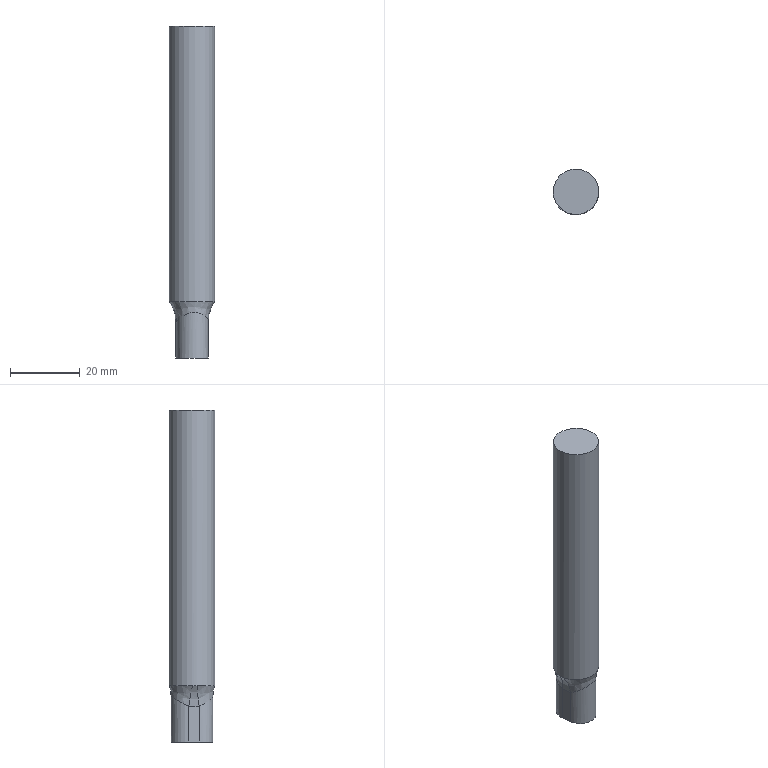Part | NX | features SPES-C 13-10-12.00-9.000 2 | 1 solid | 11 faces | box 13 x 13 x 95 mm | volume 11996 mm3 | plane 4 | spline 4 | cylinder 3 | commonest cylinder face diameters 9 x2 13 x1
STEP:
#1=CARTESIAN_POINT('',(601.161,-36.407,-10.773));
#2=VERTEX_POINT('',#1);
#3=CARTESIAN_POINT('',(601.161,-36.407,-21.));
#4=VERTEX_POINT('',#3);
#5=CARTESIAN_POINT('',(601.161,-36.407,-4.878));
#6=DIRECTION('',(0.,0.,-1.));
#7=VECTOR('',#6,1000.);
#8=LINE('',#5,#7);
#9=EDGE_CURVE('',#2,#4,#8,.T.);
#10=ORIENTED_EDGE('',*,*,#9,.F.);
#11=CARTESIAN_POINT('',(610.092,-35.294,-10.773));
#12=VERTEX_POINT('',#11);
#13=CARTESIAN_POINT('',(601.161,-36.407,-10.773));
#14=CARTESIAN_POINT('',(601.016,-35.246,-10.241));
#15=CARTESIAN_POINT('',(601.492,-33.509,-9.332));
#16=CARTESIAN_POINT('',(603.219,-31.901,-8.27));
#17=CARTESIAN_POINT('',(605.065,-31.242,-7.864));
#18=CARTESIAN_POINT('',(606.998,-31.435,-8.274));
#19=CARTESIAN_POINT('',(609.066,-32.573,-9.336));
#20=CARTESIAN_POINT('',(609.947,-34.134,-10.242));
#21=CARTESIAN_POINT('',(610.092,-35.294,-10.773));
#22=B_SPLINE_CURVE_WITH_KNOTS('',3,(#13,#14,#15,#16,#17,#18,#19,#20,#21),.UNSPECIFIED.,.F.,.F.,(4,1,1,1,1,1,4),(0.,0.003836,0.005754,0.007673,0.009591,0.01151,0.01535),.UNSPECIFIED.);
#23=EDGE_CURVE('',#2,#12,#22,.T.);
#24=ORIENTED_EDGE('',*,*,#23,.T.);
#25=CARTESIAN_POINT('',(610.092,-35.294,-21.));
#26=VERTEX_POINT('',#25);
#27=CARTESIAN_POINT('',(610.092,-35.294,-4.878));
#28=DIRECTION('',(0.,0.,-1.));
#29=VECTOR('',#28,1000.);
#30=LINE('',#27,#29);
#31=EDGE_CURVE('',#12,#26,#30,.T.);
#32=ORIENTED_EDGE('',*,*,#31,.T.);
#33=CARTESIAN_POINT('',(605.626,-35.851,-21.));
#34=DIRECTION('',(0.,0.,1.));
#35=DIRECTION('',(1.,0.,0.));
#36=AXIS2_PLACEMENT_3D('',#33,#34,#35);
#37=CIRCLE('',#36,4.5);
#38=EDGE_CURVE('',#26,#4,#37,.T.);
#39=ORIENTED_EDGE('',*,*,#38,.T.);
#40=EDGE_LOOP('',(#10,#24,#32,#39));
#41=FACE_BOUND('',#40,.T.);
#42=CARTESIAN_POINT('',(605.626,-35.851,-4.878));
#43=DIRECTION('',(0.,0.,-1.));
#44=DIRECTION('',(-1.,0.,0.));
#45=AXIS2_PLACEMENT_3D('',#42,#43,#44);
#46=CYLINDRICAL_SURFACE('',#45,4.5);
#47=ADVANCED_FACE('',(#41),#46,.T.);
#48=CARTESIAN_POINT('',(601.531,-39.384,-10.773));
#49=VERTEX_POINT('',#48);
#50=CARTESIAN_POINT('',(601.531,-39.384,-21.));
#51=VERTEX_POINT('',#50);
#52=CARTESIAN_POINT('',(601.531,-39.384,-4.878));
#53=DIRECTION('',(0.,0.,-1.));
#54=VECTOR('',#53,1000.);
#55=LINE('',#52,#54);
#56=EDGE_CURVE('',#49,#51,#55,.T.);
#57=ORIENTED_EDGE('',*,*,#56,.F.);
#58=CARTESIAN_POINT('',(601.531,-39.384,-10.773));
#59=CARTESIAN_POINT('',(601.408,-38.394,-10.914));
#60=CARTESIAN_POINT('',(601.284,-37.397,-10.914));
#61=CARTESIAN_POINT('',(601.161,-36.407,-10.773));
#62=B_SPLINE_CURVE_WITH_KNOTS('',3,(#58,#59,#60,#61),.UNSPECIFIED.,.F.,.F.,(4,4),(0.,0.003022),.UNSPECIFIED.);
#63=EDGE_CURVE('',#49,#2,#62,.T.);
#64=ORIENTED_EDGE('',*,*,#63,.T.);
#65=ORIENTED_EDGE('',*,*,#9,.T.);
#66=CARTESIAN_POINT('',(601.531,-39.384,-21.));
#67=DIRECTION('',(-0.1236,0.9923,0.));
#68=VECTOR('',#67,1000.);
#69=LINE('',#66,#68);
#70=EDGE_CURVE('',#51,#4,#69,.T.);
#71=ORIENTED_EDGE('',*,*,#70,.F.);
#72=EDGE_LOOP('',(#57,#64,#65,#71));
#73=FACE_BOUND('',#72,.T.);
#74=CARTESIAN_POINT('',(601.531,-39.384,-4.878));
#75=DIRECTION('',(-0.9923,-0.1236,0.));
#76=DIRECTION('',(0.1236,-0.9923,0.));
#77=AXIS2_PLACEMENT_3D('',#74,#75,#76);
#78=PLANE('',#77);
#79=ADVANCED_FACE('',(#73),#78,.T.);
#80=CARTESIAN_POINT('',(610.462,-38.271,-10.773));
#81=VERTEX_POINT('',#80);
#82=CARTESIAN_POINT('',(610.462,-38.271,-21.));
#83=VERTEX_POINT('',#82);
#84=CARTESIAN_POINT('',(610.462,-38.271,-4.878));
#85=DIRECTION('',(0.,0.,-1.));
#86=VECTOR('',#85,1000.);
#87=LINE('',#84,#86);
#88=EDGE_CURVE('',#81,#83,#87,.T.);
#89=ORIENTED_EDGE('',*,*,#88,.F.);
#90=CARTESIAN_POINT('',(610.462,-38.271,-10.773));
#91=CARTESIAN_POINT('',(610.607,-39.433,-10.241));
#92=CARTESIAN_POINT('',(610.131,-41.169,-9.332));
#93=CARTESIAN_POINT('',(608.404,-42.778,-8.27));
#94=CARTESIAN_POINT('',(606.559,-43.436,-7.864));
#95=CARTESIAN_POINT('',(604.625,-43.244,-8.274));
#96=CARTESIAN_POINT('',(602.557,-42.106,-9.336));
#97=CARTESIAN_POINT('',(601.676,-40.544,-10.242));
#98=CARTESIAN_POINT('',(601.531,-39.384,-10.773));
#99=B_SPLINE_CURVE_WITH_KNOTS('',3,(#90,#91,#92,#93,#94,#95,#96,#97,#98),.UNSPECIFIED.,.F.,.F.,(4,1,1,1,1,1,4),(0.,0.003836,0.005754,0.007673,0.009591,0.01151,0.01535),.UNSPECIFIED.);
#100=EDGE_CURVE('',#81,#49,#99,.T.);
#101=ORIENTED_EDGE('',*,*,#100,.T.);
#102=ORIENTED_EDGE('',*,*,#56,.T.);
#103=CARTESIAN_POINT('',(605.997,-38.828,-21.));
#104=DIRECTION('',(0.,0.,1.));
#105=DIRECTION('',(1.,0.,0.));
#106=AXIS2_PLACEMENT_3D('',#103,#104,#105);
#107=CIRCLE('',#106,4.5);
#108=EDGE_CURVE('',#51,#83,#107,.T.);
#109=ORIENTED_EDGE('',*,*,#108,.T.);
#110=EDGE_LOOP('',(#89,#101,#102,#109));
#111=FACE_BOUND('',#110,.T.);
#112=CARTESIAN_POINT('',(605.997,-38.828,-4.878));
#113=DIRECTION('',(0.,0.,-1.));
#114=DIRECTION('',(-1.,0.,0.));
#115=AXIS2_PLACEMENT_3D('',#112,#113,#114);
#116=CYLINDRICAL_SURFACE('',#115,4.5);
#117=ADVANCED_FACE('',(#111),#116,.T.);
#118=ORIENTED_EDGE('',*,*,#31,.F.);
#119=CARTESIAN_POINT('',(610.092,-35.294,-10.773));
#120=CARTESIAN_POINT('',(610.215,-36.284,-10.914));
#121=CARTESIAN_POINT('',(610.339,-37.281,-10.914));
#122=CARTESIAN_POINT('',(610.462,-38.271,-10.773));
#123=B_SPLINE_CURVE_WITH_KNOTS('',3,(#119,#120,#121,#122),.UNSPECIFIED.,.F.,.F.,(4,4),(0.,0.003022),.UNSPECIFIED.);
#124=EDGE_CURVE('',#12,#81,#123,.T.);
#125=ORIENTED_EDGE('',*,*,#124,.T.);
#126=ORIENTED_EDGE('',*,*,#88,.T.);
#127=CARTESIAN_POINT('',(610.462,-38.271,-21.));
#128=DIRECTION('',(-0.1236,0.9923,0.));
#129=VECTOR('',#128,1000.);
#130=LINE('',#127,#129);
#131=EDGE_CURVE('',#83,#26,#130,.T.);
#132=ORIENTED_EDGE('',*,*,#131,.T.);
#133=EDGE_LOOP('',(#118,#125,#126,#132));
#134=FACE_BOUND('',#133,.T.);
#135=CARTESIAN_POINT('',(610.462,-38.271,-4.878));
#136=DIRECTION('',(-0.9923,-0.1236,0.));
#137=DIRECTION('',(0.1236,-0.9923,0.));
#138=AXIS2_PLACEMENT_3D('',#135,#136,#137);
#139=PLANE('',#138);
#140=ADVANCED_FACE('',(#134),#139,.F.);
#141=ORIENTED_EDGE('',*,*,#38,.F.);
#142=ORIENTED_EDGE('',*,*,#131,.F.);
#143=ORIENTED_EDGE('',*,*,#108,.F.);
#144=ORIENTED_EDGE('',*,*,#70,.T.);
#145=EDGE_LOOP('',(#141,#142,#143,#144));
#146=FACE_BOUND('',#145,.T.);
#147=CARTESIAN_POINT('',(605.626,-35.851,-21.));
#148=DIRECTION('',(0.,0.,1.));
#149=DIRECTION('',(1.,0.,0.));
#150=AXIS2_PLACEMENT_3D('',#147,#148,#149);
#151=PLANE('',#150);
#152=ADVANCED_FACE('',(#146),#151,.F.);
#153=CARTESIAN_POINT('',(599.312,-37.339,74.));
#154=VERTEX_POINT('',#153);
#155=CARTESIAN_POINT('',(605.812,-37.339,74.));
#156=DIRECTION('',(0.,0.,-1.));
#157=DIRECTION('',(-1.,0.,0.));
#158=AXIS2_PLACEMENT_3D('',#155,#156,#157);
#159=CIRCLE('',#158,6.5);
#160=EDGE_CURVE('',#154,#154,#159,.T.);
#161=ORIENTED_EDGE('',*,*,#160,.F.);
#162=EDGE_LOOP('',(#161));
#163=FACE_BOUND('',#162,.T.);
#164=CARTESIAN_POINT('',(605.812,-37.339,74.));
#165=DIRECTION('',(0.,0.,1.));
#166=DIRECTION('',(1.,0.,0.));
#167=AXIS2_PLACEMENT_3D('',#164,#165,#166);
#168=PLANE('',#167);
#169=ADVANCED_FACE('',(#163),#168,.T.);
#170=ORIENTED_EDGE('',*,*,#160,.T.);
#171=EDGE_LOOP('',(#170));
#172=FACE_BOUND('',#171,.T.);
#173=CARTESIAN_POINT('',(612.31,-37.204,-4.878));
#174=VERTEX_POINT('',#173);
#175=CARTESIAN_POINT('',(612.145,-35.876,-4.878));
#176=VERTEX_POINT('',#175);
#177=CARTESIAN_POINT('',(605.812,-37.339,-4.878));
#178=DIRECTION('',(0.,0.,1.));
#179=DIRECTION('',(1.,0.,0.));
#180=AXIS2_PLACEMENT_3D('',#177,#178,#179);
#181=CIRCLE('',#180,6.5);
#182=EDGE_CURVE('',#174,#176,#181,.T.);
#183=ORIENTED_EDGE('',*,*,#182,.T.);
#184=CARTESIAN_POINT('',(599.313,-37.475,-4.878));
#185=VERTEX_POINT('',#184);
#186=CARTESIAN_POINT('',(605.812,-37.339,-4.878));
#187=DIRECTION('',(0.,0.,1.));
#188=DIRECTION('',(1.,0.,0.));
#189=AXIS2_PLACEMENT_3D('',#186,#187,#188);
#190=CIRCLE('',#189,6.5);
#191=EDGE_CURVE('',#176,#185,#190,.T.);
#192=ORIENTED_EDGE('',*,*,#191,.T.);
#193=CARTESIAN_POINT('',(599.478,-38.802,-4.878));
#194=VERTEX_POINT('',#193);
#195=CARTESIAN_POINT('',(605.812,-37.339,-4.878));
#196=DIRECTION('',(0.,0.,1.));
#197=DIRECTION('',(1.,0.,0.));
#198=AXIS2_PLACEMENT_3D('',#195,#196,#197);
#199=CIRCLE('',#198,6.5);
#200=EDGE_CURVE('',#185,#194,#199,.T.);
#201=ORIENTED_EDGE('',*,*,#200,.T.);
#202=CARTESIAN_POINT('',(605.812,-37.339,-4.878));
#203=DIRECTION('',(0.,0.,1.));
#204=DIRECTION('',(1.,0.,0.));
#205=AXIS2_PLACEMENT_3D('',#202,#203,#204);
#206=CIRCLE('',#205,6.5);
#207=EDGE_CURVE('',#194,#174,#206,.T.);
#208=ORIENTED_EDGE('',*,*,#207,.T.);
#209=EDGE_LOOP('',(#183,#192,#201,#208));
#210=FACE_BOUND('',#209,.T.);
#211=CARTESIAN_POINT('',(605.812,-37.339,-4.878));
#212=DIRECTION('',(0.,0.,1.));
#213=DIRECTION('',(1.,0.,0.));
#214=AXIS2_PLACEMENT_3D('',#211,#212,#213);
#215=CYLINDRICAL_SURFACE('',#214,6.5);
#216=ADVANCED_FACE('',(#172,#210),#215,.T.);
#217=CARTESIAN_POINT('',(620.015,-34.058,-10.773));
#218=DIRECTION('',(0.1224,-0.9826,-0.1396));
#219=DIRECTION('',(0.,0.1407,-0.9901));
#220=AXIS2_PLACEMENT_3D('',#217,#218,#219);
#221=CIRCLE('',#220,10.);
#222=EDGE_CURVE('',#176,#12,#221,.T.);
#223=ORIENTED_EDGE('',*,*,#222,.F.);
#224=ORIENTED_EDGE('',*,*,#182,.F.);
#225=CARTESIAN_POINT('',(620.386,-37.035,-10.773));
#226=DIRECTION('',(0.1224,-0.9826,0.1396));
#227=DIRECTION('',(0.,-0.1407,-0.9901));
#228=AXIS2_PLACEMENT_3D('',#225,#226,#227);
#229=CIRCLE('',#228,10.);
#230=EDGE_CURVE('',#81,#174,#229,.F.);
#231=ORIENTED_EDGE('',*,*,#230,.F.);
#232=ORIENTED_EDGE('',*,*,#124,.F.);
#233=EDGE_LOOP('',(#223,#224,#231,#232));
#234=FACE_BOUND('',#233,.T.);
#235=CARTESIAN_POINT('',(612.31,-37.204,-4.878));
#236=CARTESIAN_POINT('',(610.405,-37.814,-7.504));
#237=CARTESIAN_POINT('',(610.462,-38.271,-10.773));
#238=CARTESIAN_POINT('',(612.301,-36.762,-4.878));
#239=CARTESIAN_POINT('',(610.32,-37.13,-7.558));
#240=CARTESIAN_POINT('',(610.339,-37.284,-10.913));
#241=CARTESIAN_POINT('',(612.244,-36.306,-4.878));
#242=CARTESIAN_POINT('',(610.234,-36.434,-7.558));
#243=CARTESIAN_POINT('',(610.214,-36.281,-10.913));
#244=CARTESIAN_POINT('',(612.145,-35.876,-4.878));
#245=CARTESIAN_POINT('',(610.149,-35.752,-7.504));
#246=CARTESIAN_POINT('',(610.092,-35.294,-10.773));
#247=(BOUNDED_SURFACE()B_SPLINE_SURFACE(3,2,((#235,#236,#237),(#238,#239,#240),(#241,#242,#243),(#244,#245,#246)),.UNSPECIFIED.,.F.,.F.,.F.)B_SPLINE_SURFACE_WITH_KNOTS((4,4),(3,3),(0.009413,0.01241),(0.,1.),.PIECEWISE_BEZIER_KNOTS.)GEOMETRIC_REPRESENTATION_ITEM()RATIONAL_B_SPLINE_SURFACE(((1.,0.9496,1.),(1.,0.9484,1.),(1.,0.9484,1.),(1.,0.9496,1.)))REPRESENTATION_ITEM('')SURFACE());
#248=ADVANCED_FACE('',(#234),#247,.F.);
#249=ORIENTED_EDGE('',*,*,#230,.T.);
#250=ORIENTED_EDGE('',*,*,#207,.F.);
#251=CARTESIAN_POINT('',(591.608,-40.62,-10.773));
#252=DIRECTION('',(-0.1224,0.9826,-0.1396));
#253=DIRECTION('',(0.,0.1407,0.9901));
#254=AXIS2_PLACEMENT_3D('',#251,#252,#253);
#255=CIRCLE('',#254,10.);
#256=EDGE_CURVE('',#49,#194,#255,.F.);
#257=ORIENTED_EDGE('',*,*,#256,.F.);
#258=ORIENTED_EDGE('',*,*,#100,.F.);
#259=EDGE_LOOP('',(#249,#250,#257,#258));
#260=FACE_BOUND('',#259,.T.);
#261=CARTESIAN_POINT('',(599.478,-38.802,-4.878));
#262=CARTESIAN_POINT('',(601.475,-38.927,-7.504));
#263=CARTESIAN_POINT('',(601.531,-39.384,-10.773));
#264=CARTESIAN_POINT('',(599.859,-40.451,-4.878));
#265=CARTESIAN_POINT('',(601.5,-40.104,-7.337));
#266=CARTESIAN_POINT('',(601.678,-40.559,-10.235));
#267=CARTESIAN_POINT('',(601.368,-42.528,-4.878));
#268=CARTESIAN_POINT('',(602.289,-41.928,-6.973));
#269=CARTESIAN_POINT('',(602.616,-42.193,-9.279));
#270=CARTESIAN_POINT('',(604.263,-43.797,-4.878));
#271=CARTESIAN_POINT('',(604.565,-43.246,-6.506));
#272=CARTESIAN_POINT('',(604.754,-43.275,-8.231));
#273=CARTESIAN_POINT('',(607.433,-43.974,-4.878));
#274=CARTESIAN_POINT('',(607.252,-43.507,-6.29));
#275=CARTESIAN_POINT('',(607.183,-43.46,-7.766));
#276=CARTESIAN_POINT('',(611.086,-42.078,-4.878));
#277=CARTESIAN_POINT('',(610.27,-41.578,-6.85));
#278=CARTESIAN_POINT('',(609.943,-41.873,-8.953));
#279=CARTESIAN_POINT('',(612.345,-38.877,-4.878));
#280=CARTESIAN_POINT('',(610.667,-38.95,-7.339));
#281=CARTESIAN_POINT('',(610.607,-39.434,-10.241));
#282=CARTESIAN_POINT('',(612.31,-37.204,-4.878));
#283=CARTESIAN_POINT('',(610.405,-37.814,-7.504));
#284=CARTESIAN_POINT('',(610.462,-38.271,-10.773));
#285=(BOUNDED_SURFACE()B_SPLINE_SURFACE(3,2,((#261,#262,#263),(#264,#265,#266),(#267,#268,#269),(#270,#271,#272),(#273,#274,#275),(#276,#277,#278),(#279,#280,#281),(#282,#283,#284)),.UNSPECIFIED.,.F.,.F.,.F.)B_SPLINE_SURFACE_WITH_KNOTS((4,1,1,1,1,4),(3,3),(0.02407,0.0355,0.04122,0.04693,0.05836,0.06979),(0.,1.),.UNSPECIFIED.)GEOMETRIC_REPRESENTATION_ITEM()RATIONAL_B_SPLINE_SURFACE(((1.,0.9496,1.),(1.,0.9599,1.),(1.,0.9745,1.),(1.,0.9855,1.),(1.,0.9894,1.),(1.,0.9795,1.),(1.,0.9598,1.),(1.,0.9496,1.)))REPRESENTATION_ITEM('')SURFACE());
#286=ADVANCED_FACE('',(#260),#285,.F.);
#287=ORIENTED_EDGE('',*,*,#222,.T.);
#288=ORIENTED_EDGE('',*,*,#23,.F.);
#289=CARTESIAN_POINT('',(591.237,-37.643,-10.773));
#290=DIRECTION('',(-0.1224,0.9826,0.1396));
#291=DIRECTION('',(0.,-0.1407,0.9901));
#292=AXIS2_PLACEMENT_3D('',#289,#290,#291);
#293=CIRCLE('',#292,10.);
#294=EDGE_CURVE('',#185,#2,#293,.T.);
#295=ORIENTED_EDGE('',*,*,#294,.F.);
#296=ORIENTED_EDGE('',*,*,#191,.F.);
#297=EDGE_LOOP('',(#287,#288,#295,#296));
#298=FACE_BOUND('',#297,.T.);
#299=CARTESIAN_POINT('',(612.145,-35.876,-4.878));
#300=CARTESIAN_POINT('',(610.149,-35.752,-7.504));
#301=CARTESIAN_POINT('',(610.092,-35.294,-10.773));
#302=CARTESIAN_POINT('',(611.764,-34.228,-4.878));
#303=CARTESIAN_POINT('',(610.123,-34.575,-7.337));
#304=CARTESIAN_POINT('',(609.945,-34.12,-10.235));
#305=CARTESIAN_POINT('',(610.255,-32.151,-4.878));
#306=CARTESIAN_POINT('',(609.334,-32.751,-6.973));
#307=CARTESIAN_POINT('',(609.007,-32.485,-9.279));
#308=CARTESIAN_POINT('',(607.36,-30.882,-4.878));
#309=CARTESIAN_POINT('',(607.058,-31.432,-6.506));
#310=CARTESIAN_POINT('',(606.869,-31.403,-8.231));
#311=CARTESIAN_POINT('',(604.19,-30.704,-4.878));
#312=CARTESIAN_POINT('',(604.371,-31.171,-6.29));
#313=CARTESIAN_POINT('',(604.441,-31.218,-7.766));
#314=CARTESIAN_POINT('',(600.537,-32.601,-4.878));
#315=CARTESIAN_POINT('',(601.353,-33.101,-6.85));
#316=CARTESIAN_POINT('',(601.68,-32.806,-8.953));
#317=CARTESIAN_POINT('',(599.278,-35.801,-4.878));
#318=CARTESIAN_POINT('',(600.956,-35.729,-7.339));
#319=CARTESIAN_POINT('',(601.016,-35.245,-10.241));
#320=CARTESIAN_POINT('',(599.313,-37.475,-4.878));
#321=CARTESIAN_POINT('',(601.218,-36.865,-7.504));
#322=CARTESIAN_POINT('',(601.161,-36.407,-10.773));
#323=(BOUNDED_SURFACE()B_SPLINE_SURFACE(3,2,((#299,#300,#301),(#302,#303,#304),(#305,#306,#307),(#308,#309,#310),(#311,#312,#313),(#314,#315,#316),(#317,#318,#319),(#320,#321,#322)),.UNSPECIFIED.,.F.,.F.,.F.)B_SPLINE_SURFACE_WITH_KNOTS((4,1,1,1,1,4),(3,3),(0.02407,0.0355,0.04122,0.04693,0.05836,0.06979),(0.,1.),.UNSPECIFIED.)GEOMETRIC_REPRESENTATION_ITEM()RATIONAL_B_SPLINE_SURFACE(((1.,0.9496,1.),(1.,0.9599,1.),(1.,0.9745,1.),(1.,0.9855,1.),(1.,0.9894,1.),(1.,0.9795,1.),(1.,0.9598,1.),(1.,0.9496,1.)))REPRESENTATION_ITEM('')SURFACE());
#324=ADVANCED_FACE('',(#298),#323,.F.);
#325=ORIENTED_EDGE('',*,*,#256,.T.);
#326=ORIENTED_EDGE('',*,*,#200,.F.);
#327=ORIENTED_EDGE('',*,*,#294,.T.);
#328=ORIENTED_EDGE('',*,*,#63,.F.);
#329=EDGE_LOOP('',(#325,#326,#327,#328));
#330=FACE_BOUND('',#329,.T.);
#331=CARTESIAN_POINT('',(599.313,-37.475,-4.878));
#332=CARTESIAN_POINT('',(601.218,-36.865,-7.504));
#333=CARTESIAN_POINT('',(601.161,-36.407,-10.773));
#334=CARTESIAN_POINT('',(599.322,-37.916,-4.878));
#335=CARTESIAN_POINT('',(601.303,-37.548,-7.558));
#336=CARTESIAN_POINT('',(601.284,-37.395,-10.913));
#337=CARTESIAN_POINT('',(599.379,-38.373,-4.878));
#338=CARTESIAN_POINT('',(601.389,-38.244,-7.558));
#339=CARTESIAN_POINT('',(601.409,-38.398,-10.913));
#340=CARTESIAN_POINT('',(599.478,-38.802,-4.878));
#341=CARTESIAN_POINT('',(601.475,-38.927,-7.504));
#342=CARTESIAN_POINT('',(601.531,-39.384,-10.773));
#343=(BOUNDED_SURFACE()B_SPLINE_SURFACE(3,2,((#331,#332,#333),(#334,#335,#336),(#337,#338,#339),(#340,#341,#342)),.UNSPECIFIED.,.F.,.F.,.F.)B_SPLINE_SURFACE_WITH_KNOTS((4,4),(3,3),(0.009413,0.01241),(0.,1.),.PIECEWISE_BEZIER_KNOTS.)GEOMETRIC_REPRESENTATION_ITEM()RATIONAL_B_SPLINE_SURFACE(((1.,0.9496,1.),(1.,0.9484,1.),(1.,0.9484,1.),(1.,0.9496,1.)))REPRESENTATION_ITEM('')SURFACE());
#344=ADVANCED_FACE('',(#330),#343,.F.);
#345=CLOSED_SHELL('',(#47,#79,#117,#140,#152,#169,#216,#248,#286,#324,#344));
#346=MANIFOLD_SOLID_BREP('',#345);
#347=(LENGTH_UNIT()NAMED_UNIT(*)SI_UNIT(.MILLI.,.METRE.));
#348=UNCERTAINTY_MEASURE_WITH_UNIT(LENGTH_MEASURE(0.0508),#347,'','');
#349=(NAMED_UNIT(*)PLANE_ANGLE_UNIT()SI_UNIT($,.RADIAN.));
#350=(NAMED_UNIT(*)SI_UNIT($,.STERADIAN.)SOLID_ANGLE_UNIT());
#351=(GEOMETRIC_REPRESENTATION_CONTEXT(3)GLOBAL_UNCERTAINTY_ASSIGNED_CONTEXT((#348))GLOBAL_UNIT_ASSIGNED_CONTEXT((#347,#349,#350))REPRESENTATION_CONTEXT('',''));
#352=ADVANCED_BREP_SHAPE_REPRESENTATION('',(#346),#351);